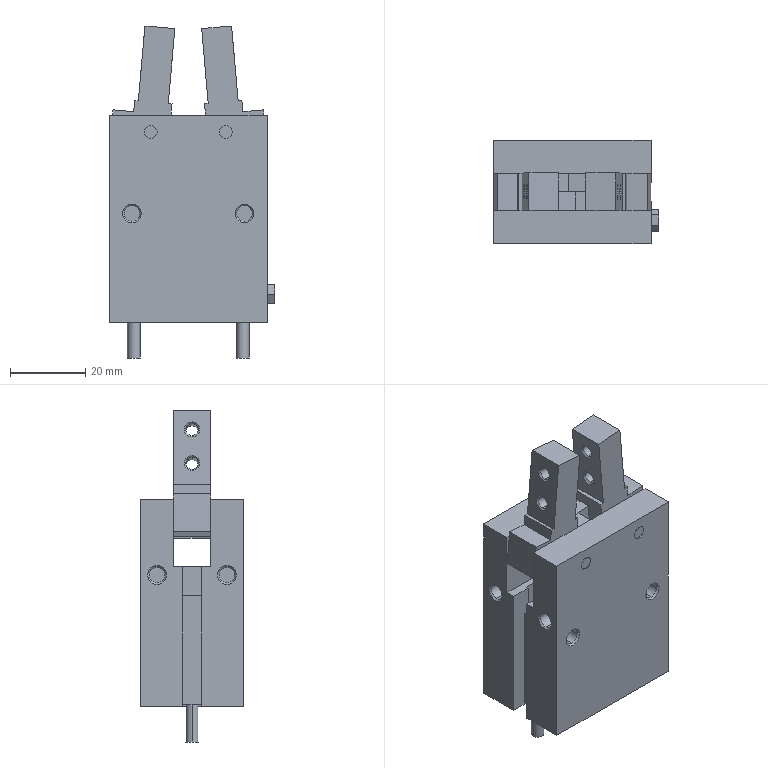Part | STEP file | 手指气缸-2 | 1 solid | 182 faces | box 44 x 27.6 x 88.442 mm | volume 60237 mm3 | plane 104 | cylinder 42 | cone 36 | commonest cylinder face diameters 4.13 x20 3.4 x12 3.24 x8 21 x2